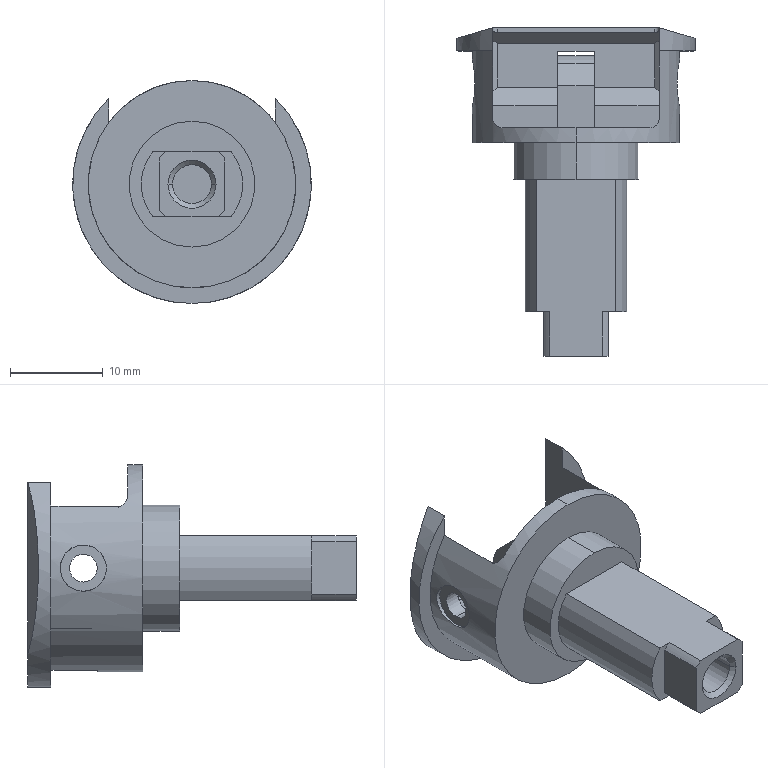Part | STEP file | _X2_751F4E45_X0_MS731-1_X2_8F_5 | 1 solid | 66 faces | box 25.8 x 35.5 x 24.1 mm | volume 3742 mm3 | plane 36 | cylinder 28 | cone 2 | commonest cylinder face diameters 3 x6 5 x4 9 x4 1 x2 2 x2 4.2 x2